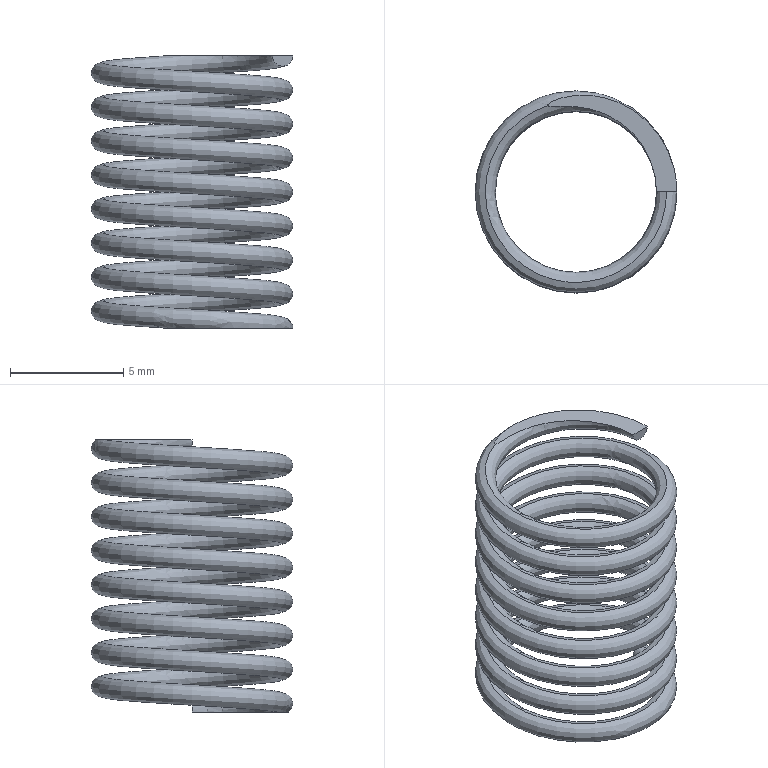Part | SolidWorks | features ICE 2, Helix 1, Sweep 1 | 1 solid | 6 faces | box 8.9 x 8.9 x 12 mm | volume 125.858 mm3 | plane 4 | spline 2